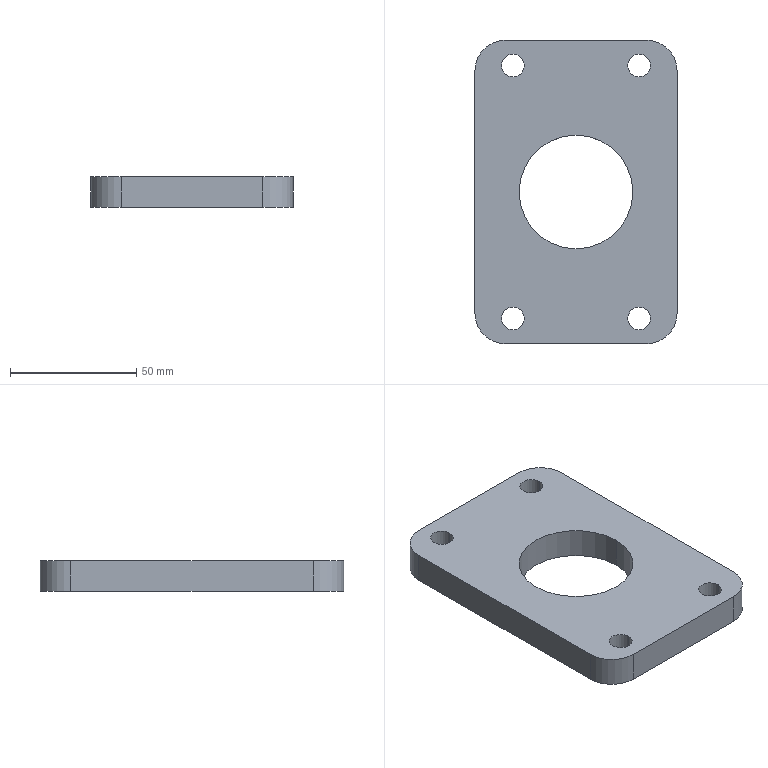Part | SolidWorks | features BaseBody 1 | 1 solid | 20 faces | box 80 x 120 x 12 mm | volume 91578 mm3 | cylinder 14 | plane 6 | commonest cylinder face diameters 9 x8 24 x4 45 x2
STEP:
#1=CARTESIAN_POINT('',(264.5,50.,-47.879));
#2=VERTEX_POINT('',#1);
#3=CARTESIAN_POINT('',(255.5,50.,-47.879));
#4=VERTEX_POINT('',#3);
#5=CARTESIAN_POINT('',(260.,50.,-47.879));
#6=DIRECTION('',(0.,0.,-1.));
#7=DIRECTION('',(-1.,0.,0.));
#8=AXIS2_PLACEMENT_3D('',#5,#6,#7);
#9=CIRCLE('',#8,4.5);
#10=EDGE_CURVE('',#2,#4,#9,.T.);
#11=ORIENTED_EDGE('',*,*,#10,.F.);
#12=CARTESIAN_POINT('',(264.5,50.,-59.879));
#13=VERTEX_POINT('',#12);
#14=CARTESIAN_POINT('',(264.5,50.,-59.879));
#15=DIRECTION('',(0.,0.,-1.));
#16=VECTOR('',#15,1000.);
#17=LINE('',#14,#16);
#18=EDGE_CURVE('',#2,#13,#17,.T.);
#19=ORIENTED_EDGE('',*,*,#18,.T.);
#20=CARTESIAN_POINT('',(255.5,50.,-59.879));
#21=VERTEX_POINT('',#20);
#22=CARTESIAN_POINT('',(260.,50.,-59.879));
#23=DIRECTION('',(0.,0.,-1.));
#24=DIRECTION('',(-1.,0.,0.));
#25=AXIS2_PLACEMENT_3D('',#22,#23,#24);
#26=CIRCLE('',#25,4.5);
#27=EDGE_CURVE('',#13,#21,#26,.T.);
#28=ORIENTED_EDGE('',*,*,#27,.T.);
#29=CARTESIAN_POINT('',(255.5,50.,-59.879));
#30=DIRECTION('',(0.,0.,-1.));
#31=VECTOR('',#30,1000.);
#32=LINE('',#29,#31);
#33=EDGE_CURVE('',#4,#21,#32,.T.);
#34=ORIENTED_EDGE('',*,*,#33,.F.);
#35=EDGE_LOOP('',(#11,#19,#28,#34));
#36=FACE_OUTER_BOUND('',#35,.T.);
#37=CARTESIAN_POINT('',(260.,50.,-59.879));
#38=DIRECTION('',(0.,0.,-1.));
#39=DIRECTION('',(-1.,0.,0.));
#40=AXIS2_PLACEMENT_3D('',#37,#38,#39);
#41=CYLINDRICAL_SURFACE('',#40,4.5);
#42=ADVANCED_FACE('',(#36),#41,.F.);
#43=CARTESIAN_POINT('',(214.5,50.,-47.879));
#44=VERTEX_POINT('',#43);
#45=CARTESIAN_POINT('',(205.5,50.,-47.879));
#46=VERTEX_POINT('',#45);
#47=CARTESIAN_POINT('',(210.,50.,-47.879));
#48=DIRECTION('',(0.,0.,-1.));
#49=DIRECTION('',(-1.,0.,0.));
#50=AXIS2_PLACEMENT_3D('',#47,#48,#49);
#51=CIRCLE('',#50,4.5);
#52=EDGE_CURVE('',#44,#46,#51,.T.);
#53=ORIENTED_EDGE('',*,*,#52,.F.);
#54=CARTESIAN_POINT('',(214.5,50.,-59.879));
#55=VERTEX_POINT('',#54);
#56=CARTESIAN_POINT('',(214.5,50.,-59.879));
#57=DIRECTION('',(0.,0.,-1.));
#58=VECTOR('',#57,1000.);
#59=LINE('',#56,#58);
#60=EDGE_CURVE('',#44,#55,#59,.T.);
#61=ORIENTED_EDGE('',*,*,#60,.T.);
#62=CARTESIAN_POINT('',(205.5,50.,-59.879));
#63=VERTEX_POINT('',#62);
#64=CARTESIAN_POINT('',(210.,50.,-59.879));
#65=DIRECTION('',(0.,0.,-1.));
#66=DIRECTION('',(-1.,0.,0.));
#67=AXIS2_PLACEMENT_3D('',#64,#65,#66);
#68=CIRCLE('',#67,4.5);
#69=EDGE_CURVE('',#55,#63,#68,.T.);
#70=ORIENTED_EDGE('',*,*,#69,.T.);
#71=CARTESIAN_POINT('',(205.5,50.,-59.879));
#72=DIRECTION('',(0.,0.,-1.));
#73=VECTOR('',#72,1000.);
#74=LINE('',#71,#73);
#75=EDGE_CURVE('',#46,#63,#74,.T.);
#76=ORIENTED_EDGE('',*,*,#75,.F.);
#77=EDGE_LOOP('',(#53,#61,#70,#76));
#78=FACE_OUTER_BOUND('',#77,.T.);
#79=CARTESIAN_POINT('',(210.,50.,-59.879));
#80=DIRECTION('',(0.,0.,-1.));
#81=DIRECTION('',(-1.,0.,0.));
#82=AXIS2_PLACEMENT_3D('',#79,#80,#81);
#83=CYLINDRICAL_SURFACE('',#82,4.5);
#84=ADVANCED_FACE('',(#78),#83,.F.);
#85=CARTESIAN_POINT('',(257.5,0.,-47.879));
#86=VERTEX_POINT('',#85);
#87=CARTESIAN_POINT('',(212.5,0.,-47.879));
#88=VERTEX_POINT('',#87);
#89=CARTESIAN_POINT('',(235.,0.,-47.879));
#90=DIRECTION('',(0.,0.,-1.));
#91=DIRECTION('',(-1.,0.,0.));
#92=AXIS2_PLACEMENT_3D('',#89,#90,#91);
#93=CIRCLE('',#92,22.5);
#94=EDGE_CURVE('',#86,#88,#93,.T.);
#95=ORIENTED_EDGE('',*,*,#94,.F.);
#96=CARTESIAN_POINT('',(257.5,0.,-59.879));
#97=VERTEX_POINT('',#96);
#98=CARTESIAN_POINT('',(257.5,0.,-59.879));
#99=DIRECTION('',(0.,0.,-1.));
#100=VECTOR('',#99,1000.);
#101=LINE('',#98,#100);
#102=EDGE_CURVE('',#86,#97,#101,.T.);
#103=ORIENTED_EDGE('',*,*,#102,.T.);
#104=CARTESIAN_POINT('',(212.5,0.,-59.879));
#105=VERTEX_POINT('',#104);
#106=CARTESIAN_POINT('',(235.,0.,-59.879));
#107=DIRECTION('',(0.,0.,-1.));
#108=DIRECTION('',(-1.,0.,0.));
#109=AXIS2_PLACEMENT_3D('',#106,#107,#108);
#110=CIRCLE('',#109,22.5);
#111=EDGE_CURVE('',#97,#105,#110,.T.);
#112=ORIENTED_EDGE('',*,*,#111,.T.);
#113=CARTESIAN_POINT('',(212.5,0.,-59.879));
#114=DIRECTION('',(0.,0.,-1.));
#115=VECTOR('',#114,1000.);
#116=LINE('',#113,#115);
#117=EDGE_CURVE('',#88,#105,#116,.T.);
#118=ORIENTED_EDGE('',*,*,#117,.F.);
#119=EDGE_LOOP('',(#95,#103,#112,#118));
#120=FACE_OUTER_BOUND('',#119,.T.);
#121=CARTESIAN_POINT('',(235.,0.,-59.879));
#122=DIRECTION('',(0.,0.,-1.));
#123=DIRECTION('',(-1.,0.,0.));
#124=AXIS2_PLACEMENT_3D('',#121,#122,#123);
#125=CYLINDRICAL_SURFACE('',#124,22.5);
#126=ADVANCED_FACE('',(#120),#125,.F.);
#127=CARTESIAN_POINT('',(264.5,-50.,-47.879));
#128=VERTEX_POINT('',#127);
#129=CARTESIAN_POINT('',(255.5,-50.,-47.879));
#130=VERTEX_POINT('',#129);
#131=CARTESIAN_POINT('',(260.,-50.,-47.879));
#132=DIRECTION('',(0.,0.,-1.));
#133=DIRECTION('',(-1.,0.,0.));
#134=AXIS2_PLACEMENT_3D('',#131,#132,#133);
#135=CIRCLE('',#134,4.5);
#136=EDGE_CURVE('',#128,#130,#135,.T.);
#137=ORIENTED_EDGE('',*,*,#136,.F.);
#138=CARTESIAN_POINT('',(264.5,-50.,-59.879));
#139=VERTEX_POINT('',#138);
#140=CARTESIAN_POINT('',(264.5,-50.,-59.879));
#141=DIRECTION('',(0.,0.,-1.));
#142=VECTOR('',#141,1000.);
#143=LINE('',#140,#142);
#144=EDGE_CURVE('',#128,#139,#143,.T.);
#145=ORIENTED_EDGE('',*,*,#144,.T.);
#146=CARTESIAN_POINT('',(255.5,-50.,-59.879));
#147=VERTEX_POINT('',#146);
#148=CARTESIAN_POINT('',(260.,-50.,-59.879));
#149=DIRECTION('',(0.,0.,-1.));
#150=DIRECTION('',(-1.,0.,0.));
#151=AXIS2_PLACEMENT_3D('',#148,#149,#150);
#152=CIRCLE('',#151,4.5);
#153=EDGE_CURVE('',#139,#147,#152,.T.);
#154=ORIENTED_EDGE('',*,*,#153,.T.);
#155=CARTESIAN_POINT('',(255.5,-50.,-59.879));
#156=DIRECTION('',(0.,0.,-1.));
#157=VECTOR('',#156,1000.);
#158=LINE('',#155,#157);
#159=EDGE_CURVE('',#130,#147,#158,.T.);
#160=ORIENTED_EDGE('',*,*,#159,.F.);
#161=EDGE_LOOP('',(#137,#145,#154,#160));
#162=FACE_OUTER_BOUND('',#161,.T.);
#163=CARTESIAN_POINT('',(260.,-50.,-59.879));
#164=DIRECTION('',(0.,0.,-1.));
#165=DIRECTION('',(-1.,0.,0.));
#166=AXIS2_PLACEMENT_3D('',#163,#164,#165);
#167=CYLINDRICAL_SURFACE('',#166,4.5);
#168=ADVANCED_FACE('',(#162),#167,.F.);
#169=CARTESIAN_POINT('',(214.5,-50.,-47.879));
#170=VERTEX_POINT('',#169);
#171=CARTESIAN_POINT('',(205.5,-50.,-47.879));
#172=VERTEX_POINT('',#171);
#173=CARTESIAN_POINT('',(210.,-50.,-47.879));
#174=DIRECTION('',(0.,0.,-1.));
#175=DIRECTION('',(-1.,0.,0.));
#176=AXIS2_PLACEMENT_3D('',#173,#174,#175);
#177=CIRCLE('',#176,4.5);
#178=EDGE_CURVE('',#170,#172,#177,.T.);
#179=ORIENTED_EDGE('',*,*,#178,.F.);
#180=CARTESIAN_POINT('',(214.5,-50.,-59.879));
#181=VERTEX_POINT('',#180);
#182=CARTESIAN_POINT('',(214.5,-50.,-59.879));
#183=DIRECTION('',(0.,0.,-1.));
#184=VECTOR('',#183,1000.);
#185=LINE('',#182,#184);
#186=EDGE_CURVE('',#170,#181,#185,.T.);
#187=ORIENTED_EDGE('',*,*,#186,.T.);
#188=CARTESIAN_POINT('',(205.5,-50.,-59.879));
#189=VERTEX_POINT('',#188);
#190=CARTESIAN_POINT('',(210.,-50.,-59.879));
#191=DIRECTION('',(0.,0.,-1.));
#192=DIRECTION('',(-1.,0.,0.));
#193=AXIS2_PLACEMENT_3D('',#190,#191,#192);
#194=CIRCLE('',#193,4.5);
#195=EDGE_CURVE('',#181,#189,#194,.T.);
#196=ORIENTED_EDGE('',*,*,#195,.T.);
#197=CARTESIAN_POINT('',(205.5,-50.,-59.879));
#198=DIRECTION('',(0.,0.,-1.));
#199=VECTOR('',#198,1000.);
#200=LINE('',#197,#199);
#201=EDGE_CURVE('',#172,#189,#200,.T.);
#202=ORIENTED_EDGE('',*,*,#201,.F.);
#203=EDGE_LOOP('',(#179,#187,#196,#202));
#204=FACE_OUTER_BOUND('',#203,.T.);
#205=CARTESIAN_POINT('',(210.,-50.,-59.879));
#206=DIRECTION('',(0.,0.,-1.));
#207=DIRECTION('',(-1.,0.,0.));
#208=AXIS2_PLACEMENT_3D('',#205,#206,#207);
#209=CYLINDRICAL_SURFACE('',#208,4.5);
#210=ADVANCED_FACE('',(#204),#209,.F.);
#211=CARTESIAN_POINT('',(195.,-48.,-59.879));
#212=VERTEX_POINT('',#211);
#213=CARTESIAN_POINT('',(207.,-60.,-59.879));
#214=VERTEX_POINT('',#213);
#215=CARTESIAN_POINT('',(207.,-48.,-59.879));
#216=DIRECTION('',(0.,0.,1.));
#217=DIRECTION('',(-1.,0.,0.));
#218=AXIS2_PLACEMENT_3D('',#215,#216,#217);
#219=CIRCLE('',#218,12.);
#220=EDGE_CURVE('',#212,#214,#219,.T.);
#221=ORIENTED_EDGE('',*,*,#220,.F.);
#222=CARTESIAN_POINT('',(195.,48.,-59.879));
#223=VERTEX_POINT('',#222);
#224=CARTESIAN_POINT('',(195.,0.,-59.879));
#225=DIRECTION('',(0.,-1.,0.));
#226=VECTOR('',#225,1000.);
#227=LINE('',#224,#226);
#228=EDGE_CURVE('',#223,#212,#227,.T.);
#229=ORIENTED_EDGE('',*,*,#228,.F.);
#230=CARTESIAN_POINT('',(207.,60.,-59.879));
#231=VERTEX_POINT('',#230);
#232=CARTESIAN_POINT('',(207.,48.,-59.879));
#233=DIRECTION('',(0.,0.,1.));
#234=DIRECTION('',(-1.,0.,0.));
#235=AXIS2_PLACEMENT_3D('',#232,#233,#234);
#236=CIRCLE('',#235,12.);
#237=EDGE_CURVE('',#231,#223,#236,.T.);
#238=ORIENTED_EDGE('',*,*,#237,.F.);
#239=CARTESIAN_POINT('',(263.,60.,-59.879));
#240=VERTEX_POINT('',#239);
#241=CARTESIAN_POINT('',(235.,60.,-59.879));
#242=DIRECTION('',(-1.,0.,0.));
#243=VECTOR('',#242,1000.);
#244=LINE('',#241,#243);
#245=EDGE_CURVE('',#240,#231,#244,.T.);
#246=ORIENTED_EDGE('',*,*,#245,.F.);
#247=CARTESIAN_POINT('',(275.,48.,-59.879));
#248=VERTEX_POINT('',#247);
#249=CARTESIAN_POINT('',(263.,48.,-59.879));
#250=DIRECTION('',(0.,0.,1.));
#251=DIRECTION('',(-1.,0.,0.));
#252=AXIS2_PLACEMENT_3D('',#249,#250,#251);
#253=CIRCLE('',#252,12.);
#254=EDGE_CURVE('',#248,#240,#253,.T.);
#255=ORIENTED_EDGE('',*,*,#254,.F.);
#256=CARTESIAN_POINT('',(275.,-48.,-59.879));
#257=VERTEX_POINT('',#256);
#258=CARTESIAN_POINT('',(275.,0.,-59.879));
#259=DIRECTION('',(0.,1.,0.));
#260=VECTOR('',#259,1000.);
#261=LINE('',#258,#260);
#262=EDGE_CURVE('',#257,#248,#261,.T.);
#263=ORIENTED_EDGE('',*,*,#262,.F.);
#264=CARTESIAN_POINT('',(263.,-60.,-59.879));
#265=VERTEX_POINT('',#264);
#266=CARTESIAN_POINT('',(263.,-48.,-59.879));
#267=DIRECTION('',(0.,0.,1.));
#268=DIRECTION('',(-1.,0.,0.));
#269=AXIS2_PLACEMENT_3D('',#266,#267,#268);
#270=CIRCLE('',#269,12.);
#271=EDGE_CURVE('',#265,#257,#270,.T.);
#272=ORIENTED_EDGE('',*,*,#271,.F.);
#273=CARTESIAN_POINT('',(235.,-60.,-59.879));
#274=DIRECTION('',(1.,0.,0.));
#275=VECTOR('',#274,1000.);
#276=LINE('',#273,#275);
#277=EDGE_CURVE('',#214,#265,#276,.T.);
#278=ORIENTED_EDGE('',*,*,#277,.F.);
#279=EDGE_LOOP('',(#221,#229,#238,#246,#255,#263,#272,#278));
#280=FACE_OUTER_BOUND('',#279,.T.);
#281=CARTESIAN_POINT('',(260.,50.,-59.879));
#282=DIRECTION('',(0.,0.,-1.));
#283=DIRECTION('',(-1.,0.,0.));
#284=AXIS2_PLACEMENT_3D('',#281,#282,#283);
#285=CIRCLE('',#284,4.5);
#286=EDGE_CURVE('',#21,#13,#285,.T.);
#287=ORIENTED_EDGE('',*,*,#286,.F.);
#288=ORIENTED_EDGE('',*,*,#27,.F.);
#289=EDGE_LOOP('',(#287,#288));
#290=FACE_BOUND('',#289,.T.);
#291=CARTESIAN_POINT('',(210.,50.,-59.879));
#292=DIRECTION('',(0.,0.,-1.));
#293=DIRECTION('',(-1.,0.,0.));
#294=AXIS2_PLACEMENT_3D('',#291,#292,#293);
#295=CIRCLE('',#294,4.5);
#296=EDGE_CURVE('',#63,#55,#295,.T.);
#297=ORIENTED_EDGE('',*,*,#296,.F.);
#298=ORIENTED_EDGE('',*,*,#69,.F.);
#299=EDGE_LOOP('',(#297,#298));
#300=FACE_BOUND('',#299,.T.);
#301=CARTESIAN_POINT('',(235.,0.,-59.879));
#302=DIRECTION('',(0.,0.,-1.));
#303=DIRECTION('',(-1.,0.,0.));
#304=AXIS2_PLACEMENT_3D('',#301,#302,#303);
#305=CIRCLE('',#304,22.5);
#306=EDGE_CURVE('',#105,#97,#305,.T.);
#307=ORIENTED_EDGE('',*,*,#306,.F.);
#308=ORIENTED_EDGE('',*,*,#111,.F.);
#309=EDGE_LOOP('',(#307,#308));
#310=FACE_BOUND('',#309,.T.);
#311=CARTESIAN_POINT('',(260.,-50.,-59.879));
#312=DIRECTION('',(0.,0.,-1.));
#313=DIRECTION('',(-1.,0.,0.));
#314=AXIS2_PLACEMENT_3D('',#311,#312,#313);
#315=CIRCLE('',#314,4.5);
#316=EDGE_CURVE('',#147,#139,#315,.T.);
#317=ORIENTED_EDGE('',*,*,#316,.F.);
#318=ORIENTED_EDGE('',*,*,#153,.F.);
#319=EDGE_LOOP('',(#317,#318));
#320=FACE_BOUND('',#319,.T.);
#321=CARTESIAN_POINT('',(210.,-50.,-59.879));
#322=DIRECTION('',(0.,0.,-1.));
#323=DIRECTION('',(-1.,0.,0.));
#324=AXIS2_PLACEMENT_3D('',#321,#322,#323);
#325=CIRCLE('',#324,4.5);
#326=EDGE_CURVE('',#189,#181,#325,.T.);
#327=ORIENTED_EDGE('',*,*,#326,.F.);
#328=ORIENTED_EDGE('',*,*,#195,.F.);
#329=EDGE_LOOP('',(#327,#328));
#330=FACE_BOUND('',#329,.T.);
#331=CARTESIAN_POINT('',(235.,0.,-59.879));
#332=DIRECTION('',(0.,0.,1.));
#333=DIRECTION('',(1.,0.,0.));
#334=AXIS2_PLACEMENT_3D('',#331,#332,#333);
#335=PLANE('',#334);
#336=ADVANCED_FACE('',(#280,#290,#300,#310,#320,#330),#335,.F.);
#337=CARTESIAN_POINT('',(263.,-60.,-47.879));
#338=VERTEX_POINT('',#337);
#339=CARTESIAN_POINT('',(207.,-60.,-47.879));
#340=VERTEX_POINT('',#339);
#341=CARTESIAN_POINT('',(263.,-60.,-47.879));
#342=DIRECTION('',(-1.,0.,0.));
#343=VECTOR('',#342,1000.);
#344=LINE('',#341,#343);
#345=EDGE_CURVE('',#338,#340,#344,.T.);
#346=ORIENTED_EDGE('',*,*,#345,.T.);
#347=CARTESIAN_POINT('',(207.,-60.,-59.879));
#348=DIRECTION('',(0.,0.,-1.));
#349=VECTOR('',#348,1000.);
#350=LINE('',#347,#349);
#351=EDGE_CURVE('',#340,#214,#350,.T.);
#352=ORIENTED_EDGE('',*,*,#351,.T.);
#353=ORIENTED_EDGE('',*,*,#277,.T.);
#354=CARTESIAN_POINT('',(263.,-60.,-59.879));
#355=DIRECTION('',(0.,0.,1.));
#356=VECTOR('',#355,1000.);
#357=LINE('',#354,#356);
#358=EDGE_CURVE('',#265,#338,#357,.T.);
#359=ORIENTED_EDGE('',*,*,#358,.T.);
#360=EDGE_LOOP('',(#346,#352,#353,#359));
#361=FACE_OUTER_BOUND('',#360,.T.);
#362=CARTESIAN_POINT('',(263.,-60.,-59.879));
#363=DIRECTION('',(0.,-1.,0.));
#364=DIRECTION('',(0.,0.,-1.));
#365=AXIS2_PLACEMENT_3D('',#362,#363,#364);
#366=PLANE('',#365);
#367=ADVANCED_FACE('',(#361),#366,.T.);
#368=CARTESIAN_POINT('',(195.,-48.,-47.879));
#369=VERTEX_POINT('',#368);
#370=CARTESIAN_POINT('',(207.,-48.,-47.879));
#371=DIRECTION('',(0.,0.,-1.));
#372=DIRECTION('',(-1.,0.,0.));
#373=AXIS2_PLACEMENT_3D('',#370,#371,#372);
#374=CIRCLE('',#373,12.);
#375=EDGE_CURVE('',#340,#369,#374,.T.);
#376=ORIENTED_EDGE('',*,*,#375,.T.);
#377=CARTESIAN_POINT('',(195.,-48.,-59.879));
#378=DIRECTION('',(0.,0.,-1.));
#379=VECTOR('',#378,1000.);
#380=LINE('',#377,#379);
#381=EDGE_CURVE('',#369,#212,#380,.T.);
#382=ORIENTED_EDGE('',*,*,#381,.T.);
#383=ORIENTED_EDGE('',*,*,#220,.T.);
#384=ORIENTED_EDGE('',*,*,#351,.F.);
#385=EDGE_LOOP('',(#376,#382,#383,#384));
#386=FACE_OUTER_BOUND('',#385,.T.);
#387=CARTESIAN_POINT('',(207.,-48.,-59.879));
#388=DIRECTION('',(0.,0.,-1.));
#389=DIRECTION('',(-1.,0.,0.));
#390=AXIS2_PLACEMENT_3D('',#387,#388,#389);
#391=CYLINDRICAL_SURFACE('',#390,12.);
#392=ADVANCED_FACE('',(#386),#391,.T.);
#393=CARTESIAN_POINT('',(195.,48.,-47.879));
#394=VERTEX_POINT('',#393);
#395=CARTESIAN_POINT('',(195.,-48.,-47.879));
#396=DIRECTION('',(0.,1.,0.));
#397=VECTOR('',#396,1000.);
#398=LINE('',#395,#397);
#399=EDGE_CURVE('',#369,#394,#398,.T.);
#400=ORIENTED_EDGE('',*,*,#399,.T.);
#401=CARTESIAN_POINT('',(195.,48.,-59.879));
#402=DIRECTION('',(0.,0.,-1.));
#403=VECTOR('',#402,1000.);
#404=LINE('',#401,#403);
#405=EDGE_CURVE('',#394,#223,#404,.T.);
#406=ORIENTED_EDGE('',*,*,#405,.T.);
#407=ORIENTED_EDGE('',*,*,#228,.T.);
#408=ORIENTED_EDGE('',*,*,#381,.F.);
#409=EDGE_LOOP('',(#400,#406,#407,#408));
#410=FACE_OUTER_BOUND('',#409,.T.);
#411=CARTESIAN_POINT('',(195.,-48.,-59.879));
#412=DIRECTION('',(-1.,0.,0.));
#413=DIRECTION('',(0.,0.,1.));
#414=AXIS2_PLACEMENT_3D('',#411,#412,#413);
#415=PLANE('',#414);
#416=ADVANCED_FACE('',(#410),#415,.T.);
#417=CARTESIAN_POINT('',(207.,60.,-47.879));
#418=VERTEX_POINT('',#417);
#419=CARTESIAN_POINT('',(207.,48.,-47.879));
#420=DIRECTION('',(0.,0.,-1.));
#421=DIRECTION('',(-1.,0.,0.));
#422=AXIS2_PLACEMENT_3D('',#419,#420,#421);
#423=CIRCLE('',#422,12.);
#424=EDGE_CURVE('',#394,#418,#423,.T.);
#425=ORIENTED_EDGE('',*,*,#424,.T.);
#426=CARTESIAN_POINT('',(207.,60.,-59.879));
#427=DIRECTION('',(0.,0.,-1.));
#428=VECTOR('',#427,1000.);
#429=LINE('',#426,#428);
#430=EDGE_CURVE('',#418,#231,#429,.T.);
#431=ORIENTED_EDGE('',*,*,#430,.T.);
#432=ORIENTED_EDGE('',*,*,#237,.T.);
#433=ORIENTED_EDGE('',*,*,#405,.F.);
#434=EDGE_LOOP('',(#425,#431,#432,#433));
#435=FACE_OUTER_BOUND('',#434,.T.);
#436=CARTESIAN_POINT('',(207.,48.,-59.879));
#437=DIRECTION('',(0.,0.,-1.));
#438=DIRECTION('',(-1.,0.,0.));
#439=AXIS2_PLACEMENT_3D('',#436,#437,#438);
#440=CYLINDRICAL_SURFACE('',#439,12.);
#441=ADVANCED_FACE('',(#435),#440,.T.);
#442=CARTESIAN_POINT('',(263.,60.,-47.879));
#443=VERTEX_POINT('',#442);
#444=CARTESIAN_POINT('',(207.,60.,-47.879));
#445=DIRECTION('',(1.,0.,0.));
#446=VECTOR('',#445,1000.);
#447=LINE('',#444,#446);
#448=EDGE_CURVE('',#418,#443,#447,.T.);
#449=ORIENTED_EDGE('',*,*,#448,.T.);
#450=CARTESIAN_POINT('',(263.,60.,-59.879));
#451=DIRECTION('',(0.,0.,-1.));
#452=VECTOR('',#451,1000.);
#453=LINE('',#450,#452);
#454=EDGE_CURVE('',#443,#240,#453,.T.);
#455=ORIENTED_EDGE('',*,*,#454,.T.);
#456=ORIENTED_EDGE('',*,*,#245,.T.);
#457=ORIENTED_EDGE('',*,*,#430,.F.);
#458=EDGE_LOOP('',(#449,#455,#456,#457));
#459=FACE_OUTER_BOUND('',#458,.T.);
#460=CARTESIAN_POINT('',(207.,60.,-59.879));
#461=DIRECTION('',(0.,1.,0.));
#462=DIRECTION('',(0.,0.,1.));
#463=AXIS2_PLACEMENT_3D('',#460,#461,#462);
#464=PLANE('',#463);
#465=ADVANCED_FACE('',(#459),#464,.T.);
#466=CARTESIAN_POINT('',(275.,48.,-47.879));
#467=VERTEX_POINT('',#466);
#468=CARTESIAN_POINT('',(263.,48.,-47.879));
#469=DIRECTION('',(0.,0.,-1.));
#470=DIRECTION('',(-1.,0.,0.));
#471=AXIS2_PLACEMENT_3D('',#468,#469,#470);
#472=CIRCLE('',#471,12.);
#473=EDGE_CURVE('',#443,#467,#472,.T.);
#474=ORIENTED_EDGE('',*,*,#473,.T.);
#475=CARTESIAN_POINT('',(275.,48.,-59.879));
#476=DIRECTION('',(0.,0.,-1.));
#477=VECTOR('',#476,1000.);
#478=LINE('',#475,#477);
#479=EDGE_CURVE('',#467,#248,#478,.T.);
#480=ORIENTED_EDGE('',*,*,#479,.T.);
#481=ORIENTED_EDGE('',*,*,#254,.T.);
#482=ORIENTED_EDGE('',*,*,#454,.F.);
#483=EDGE_LOOP('',(#474,#480,#481,#482));
#484=FACE_OUTER_BOUND('',#483,.T.);
#485=CARTESIAN_POINT('',(263.,48.,-59.879));
#486=DIRECTION('',(0.,0.,-1.));
#487=DIRECTION('',(-1.,0.,0.));
#488=AXIS2_PLACEMENT_3D('',#485,#486,#487);
#489=CYLINDRICAL_SURFACE('',#488,12.);
#490=ADVANCED_FACE('',(#484),#489,.T.);
#491=CARTESIAN_POINT('',(275.,-48.,-47.879));
#492=VERTEX_POINT('',#491);
#493=CARTESIAN_POINT('',(275.,48.,-47.879));
#494=DIRECTION('',(0.,-1.,0.));
#495=VECTOR('',#494,1000.);
#496=LINE('',#493,#495);
#497=EDGE_CURVE('',#467,#492,#496,.T.);
#498=ORIENTED_EDGE('',*,*,#497,.T.);
#499=CARTESIAN_POINT('',(275.,-48.,-59.879));
#500=DIRECTION('',(0.,0.,-1.));
#501=VECTOR('',#500,1000.);
#502=LINE('',#499,#501);
#503=EDGE_CURVE('',#492,#257,#502,.T.);
#504=ORIENTED_EDGE('',*,*,#503,.T.);
#505=ORIENTED_EDGE('',*,*,#262,.T.);
#506=ORIENTED_EDGE('',*,*,#479,.F.);
#507=EDGE_LOOP('',(#498,#504,#505,#506));
#508=FACE_OUTER_BOUND('',#507,.T.);
#509=CARTESIAN_POINT('',(275.,48.,-59.879));
#510=DIRECTION('',(1.,0.,0.));
#511=DIRECTION('',(0.,0.,-1.));
#512=AXIS2_PLACEMENT_3D('',#509,#510,#511);
#513=PLANE('',#512);
#514=ADVANCED_FACE('',(#508),#513,.T.);
#515=CARTESIAN_POINT('',(263.,-48.,-47.879));
#516=DIRECTION('',(0.,0.,-1.));
#517=DIRECTION('',(-1.,0.,0.));
#518=AXIS2_PLACEMENT_3D('',#515,#516,#517);
#519=CIRCLE('',#518,12.);
#520=EDGE_CURVE('',#492,#338,#519,.T.);
#521=ORIENTED_EDGE('',*,*,#520,.T.);
#522=ORIENTED_EDGE('',*,*,#358,.F.);
#523=ORIENTED_EDGE('',*,*,#271,.T.);
#524=ORIENTED_EDGE('',*,*,#503,.F.);
#525=EDGE_LOOP('',(#521,#522,#523,#524));
#526=FACE_OUTER_BOUND('',#525,.T.);
#527=CARTESIAN_POINT('',(263.,-48.,-59.879));
#528=DIRECTION('',(0.,0.,-1.));
#529=DIRECTION('',(-1.,0.,0.));
#530=AXIS2_PLACEMENT_3D('',#527,#528,#529);
#531=CYLINDRICAL_SURFACE('',#530,12.);
#532=ADVANCED_FACE('',(#526),#531,.T.);
#533=ORIENTED_EDGE('',*,*,#18,.F.);
#534=CARTESIAN_POINT('',(260.,50.,-47.879));
#535=DIRECTION('',(0.,0.,-1.));
#536=DIRECTION('',(-1.,0.,0.));
#537=AXIS2_PLACEMENT_3D('',#534,#535,#536);
#538=CIRCLE('',#537,4.5);
#539=EDGE_CURVE('',#4,#2,#538,.T.);
#540=ORIENTED_EDGE('',*,*,#539,.F.);
#541=ORIENTED_EDGE('',*,*,#33,.T.);
#542=ORIENTED_EDGE('',*,*,#286,.T.);
#543=EDGE_LOOP('',(#533,#540,#541,#542));
#544=FACE_OUTER_BOUND('',#543,.T.);
#545=CARTESIAN_POINT('',(260.,50.,-59.879));
#546=DIRECTION('',(0.,0.,-1.));
#547=DIRECTION('',(-1.,0.,0.));
#548=AXIS2_PLACEMENT_3D('',#545,#546,#547);
#549=CYLINDRICAL_SURFACE('',#548,4.5);
#550=ADVANCED_FACE('',(#544),#549,.F.);
#551=ORIENTED_EDGE('',*,*,#60,.F.);
#552=CARTESIAN_POINT('',(210.,50.,-47.879));
#553=DIRECTION('',(0.,0.,-1.));
#554=DIRECTION('',(-1.,0.,0.));
#555=AXIS2_PLACEMENT_3D('',#552,#553,#554);
#556=CIRCLE('',#555,4.5);
#557=EDGE_CURVE('',#46,#44,#556,.T.);
#558=ORIENTED_EDGE('',*,*,#557,.F.);
#559=ORIENTED_EDGE('',*,*,#75,.T.);
#560=ORIENTED_EDGE('',*,*,#296,.T.);
#561=EDGE_LOOP('',(#551,#558,#559,#560));
#562=FACE_OUTER_BOUND('',#561,.T.);
#563=CARTESIAN_POINT('',(210.,50.,-59.879));
#564=DIRECTION('',(0.,0.,-1.));
#565=DIRECTION('',(-1.,0.,0.));
#566=AXIS2_PLACEMENT_3D('',#563,#564,#565);
#567=CYLINDRICAL_SURFACE('',#566,4.5);
#568=ADVANCED_FACE('',(#562),#567,.F.);
#569=ORIENTED_EDGE('',*,*,#102,.F.);
#570=CARTESIAN_POINT('',(235.,0.,-47.879));
#571=DIRECTION('',(0.,0.,-1.));
#572=DIRECTION('',(-1.,0.,0.));
#573=AXIS2_PLACEMENT_3D('',#570,#571,#572);
#574=CIRCLE('',#573,22.5);
#575=EDGE_CURVE('',#88,#86,#574,.T.);
#576=ORIENTED_EDGE('',*,*,#575,.F.);
#577=ORIENTED_EDGE('',*,*,#117,.T.);
#578=ORIENTED_EDGE('',*,*,#306,.T.);
#579=EDGE_LOOP('',(#569,#576,#577,#578));
#580=FACE_OUTER_BOUND('',#579,.T.);
#581=CARTESIAN_POINT('',(235.,0.,-59.879));
#582=DIRECTION('',(0.,0.,-1.));
#583=DIRECTION('',(-1.,0.,0.));
#584=AXIS2_PLACEMENT_3D('',#581,#582,#583);
#585=CYLINDRICAL_SURFACE('',#584,22.5);
#586=ADVANCED_FACE('',(#580),#585,.F.);
#587=ORIENTED_EDGE('',*,*,#144,.F.);
#588=CARTESIAN_POINT('',(260.,-50.,-47.879));
#589=DIRECTION('',(0.,0.,-1.));
#590=DIRECTION('',(-1.,0.,0.));
#591=AXIS2_PLACEMENT_3D('',#588,#589,#590);
#592=CIRCLE('',#591,4.5);
#593=EDGE_CURVE('',#130,#128,#592,.T.);
#594=ORIENTED_EDGE('',*,*,#593,.F.);
#595=ORIENTED_EDGE('',*,*,#159,.T.);
#596=ORIENTED_EDGE('',*,*,#316,.T.);
#597=EDGE_LOOP('',(#587,#594,#595,#596));
#598=FACE_OUTER_BOUND('',#597,.T.);
#599=CARTESIAN_POINT('',(260.,-50.,-59.879));
#600=DIRECTION('',(0.,0.,-1.));
#601=DIRECTION('',(-1.,0.,0.));
#602=AXIS2_PLACEMENT_3D('',#599,#600,#601);
#603=CYLINDRICAL_SURFACE('',#602,4.5);
#604=ADVANCED_FACE('',(#598),#603,.F.);
#605=ORIENTED_EDGE('',*,*,#186,.F.);
#606=CARTESIAN_POINT('',(210.,-50.,-47.879));
#607=DIRECTION('',(0.,0.,-1.));
#608=DIRECTION('',(-1.,0.,0.));
#609=AXIS2_PLACEMENT_3D('',#606,#607,#608);
#610=CIRCLE('',#609,4.5);
#611=EDGE_CURVE('',#172,#170,#610,.T.);
#612=ORIENTED_EDGE('',*,*,#611,.F.);
#613=ORIENTED_EDGE('',*,*,#201,.T.);
#614=ORIENTED_EDGE('',*,*,#326,.T.);
#615=EDGE_LOOP('',(#605,#612,#613,#614));
#616=FACE_OUTER_BOUND('',#615,.T.);
#617=CARTESIAN_POINT('',(210.,-50.,-59.879));
#618=DIRECTION('',(0.,0.,-1.));
#619=DIRECTION('',(-1.,0.,0.));
#620=AXIS2_PLACEMENT_3D('',#617,#618,#619);
#621=CYLINDRICAL_SURFACE('',#620,4.5);
#622=ADVANCED_FACE('',(#616),#621,.F.);
#623=ORIENTED_EDGE('',*,*,#448,.F.);
#624=ORIENTED_EDGE('',*,*,#424,.F.);
#625=ORIENTED_EDGE('',*,*,#399,.F.);
#626=ORIENTED_EDGE('',*,*,#375,.F.);
#627=ORIENTED_EDGE('',*,*,#345,.F.);
#628=ORIENTED_EDGE('',*,*,#520,.F.);
#629=ORIENTED_EDGE('',*,*,#497,.F.);
#630=ORIENTED_EDGE('',*,*,#473,.F.);
#631=EDGE_LOOP('',(#623,#624,#625,#626,#627,#628,#629,#630));
#632=FACE_OUTER_BOUND('',#631,.T.);
#633=ORIENTED_EDGE('',*,*,#539,.T.);
#634=ORIENTED_EDGE('',*,*,#10,.T.);
#635=EDGE_LOOP('',(#633,#634));
#636=FACE_BOUND('',#635,.T.);
#637=ORIENTED_EDGE('',*,*,#557,.T.);
#638=ORIENTED_EDGE('',*,*,#52,.T.);
#639=EDGE_LOOP('',(#637,#638));
#640=FACE_BOUND('',#639,.T.);
#641=ORIENTED_EDGE('',*,*,#575,.T.);
#642=ORIENTED_EDGE('',*,*,#94,.T.);
#643=EDGE_LOOP('',(#641,#642));
#644=FACE_BOUND('',#643,.T.);
#645=ORIENTED_EDGE('',*,*,#593,.T.);
#646=ORIENTED_EDGE('',*,*,#136,.T.);
#647=EDGE_LOOP('',(#645,#646));
#648=FACE_BOUND('',#647,.T.);
#649=ORIENTED_EDGE('',*,*,#611,.T.);
#650=ORIENTED_EDGE('',*,*,#178,.T.);
#651=EDGE_LOOP('',(#649,#650));
#652=FACE_BOUND('',#651,.T.);
#653=CARTESIAN_POINT('',(235.,0.,-47.879));
#654=DIRECTION('',(0.,0.,1.));
#655=DIRECTION('',(1.,0.,0.));
#656=AXIS2_PLACEMENT_3D('',#653,#654,#655);
#657=PLANE('',#656);
#658=ADVANCED_FACE('',(#632,#636,#640,#644,#648,#652),#657,.T.);
#659=CLOSED_SHELL('',(#42,#84,#126,#168,#210,#336,#367,#392,#416,#441,#465,#490,#514,#532,#550,#568,#586,#604,#622,#658));
#660=MANIFOLD_SOLID_BREP('',#659);
#661=CARTESIAN_POINT('',(0.,0.,0.));
#662=DIRECTION('',(0.,0.,1.));
#663=DIRECTION('',(1.,0.,0.));
#664=AXIS2_PLACEMENT_3D('',#661,#662,#663);
#665=(LENGTH_UNIT()NAMED_UNIT(*)SI_UNIT(.MILLI.,.METRE.));
#666=UNCERTAINTY_MEASURE_WITH_UNIT(LENGTH_MEASURE(0.00001),#665,'','');
#667=(NAMED_UNIT(*)PLANE_ANGLE_UNIT()SI_UNIT($,.RADIAN.));
#668=(NAMED_UNIT(*)SI_UNIT($,.STERADIAN.)SOLID_ANGLE_UNIT());
#669=(GEOMETRIC_REPRESENTATION_CONTEXT(3)GLOBAL_UNCERTAINTY_ASSIGNED_CONTEXT((#666))GLOBAL_UNIT_ASSIGNED_CONTEXT((#665,#667,#668))REPRESENTATION_CONTEXT('',''));
#670=ADVANCED_BREP_SHAPE_REPRESENTATION('',(#660,#664),#669);